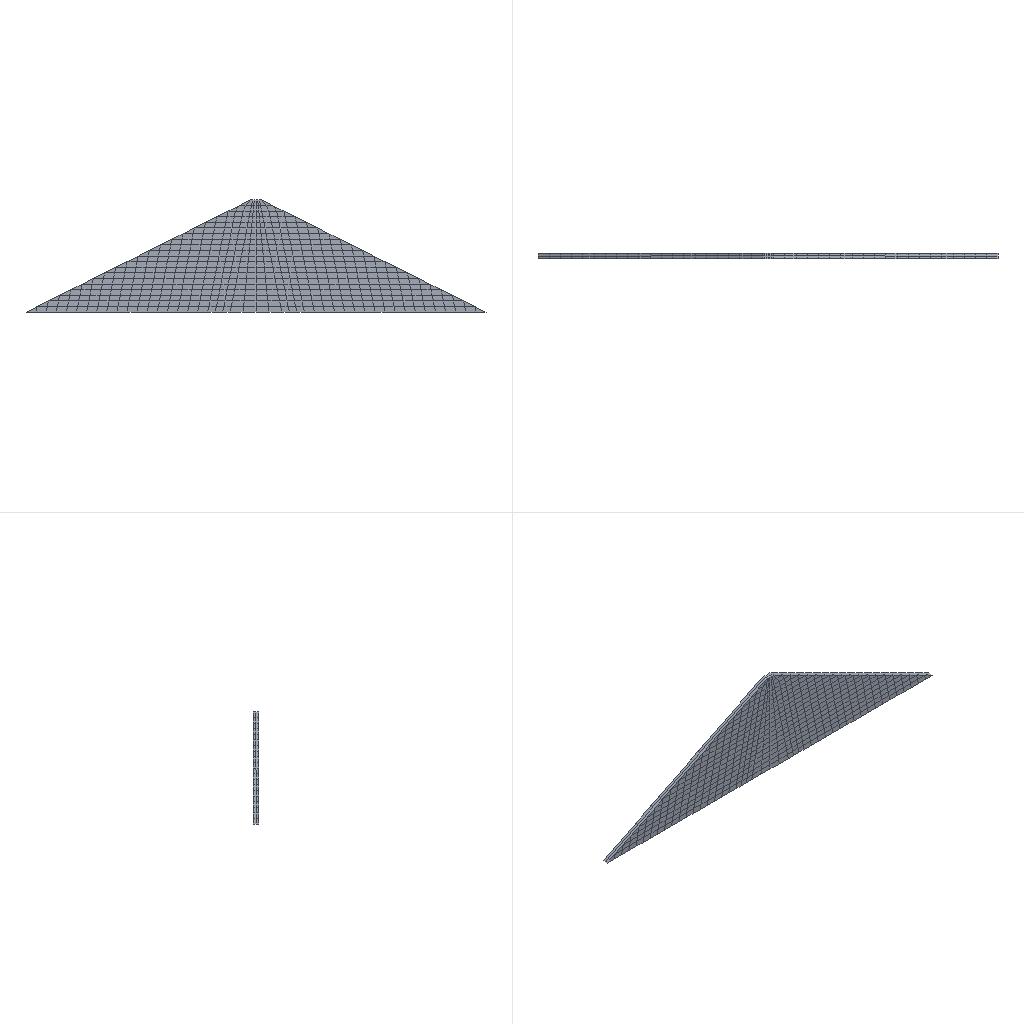Simulation study | abaqus
Set-up summary:
category,name,step,type,value,unit,region
solver,abaqus,,Abaqus/CAE 2024
units,unstated,,unstated,E= density=2 (no match)
analysis,Fill-1,,static,time_period=10
analysis,Fill-2,,static,time_period=10
analysis,Fill-3,,static,time_period=10
analysis,Fill-4,,static,time_period=10
analysis,Fiil-5,,static,time_period=10
analysis,Fill-6,,static,time_period=10
analysis,Fill-7,,static,time_period=10
analysis,Fill-8,,static,time_period=10
analysis,Fill-9,,static,time_period=10
analysis,Fill-10,,static,time_period=10
mesh,nodes,,,1701
mesh,elements,,,1080
element_type,C3D8,,,1000
element_type,C3D6,,,80
material,Core,,density,2
material,Core,,behaviors,depvar; user material
material,Rock,,density,2.2
material,Rock,,behaviors,depvar; user material
section,Rock,,solid section,,,_PickedSet30
section,Core,,solid section,,,_PickedSet29
load,,initial,initial condition solution
load,Load-1,Fill-1,gravity,"10 [dir=(0, 0, -1)]",,Part-1-1.Fill-1
load,Load-2,Fill-2,gravity,"10 [dir=(0, 0, -1)]",,Part-1-1.Fill-2
load,Load-3,Fill-3,gravity,"10 [dir=(0, 0, -1)]",,Part-1-1.Fill-3
load,Load-4,Fill-4,gravity,"10 [dir=(0, 0, -1)]",,Part-1-1.Fill-4
load,Load-5,Fiil-5,gravity,"10 [dir=(0, 0, -1)]",,Part-1-1.Fill-5
load,Load-6,Fill-6,gravity,"10 [dir=(0, 0, -1)]",,Part-1-1.Fill-6
load,Load-7,Fill-7,gravity,"10 [dir=(0, 0, -1)]",,Part-1-1.Fill-7
load,Load-8,Fill-8,gravity,"10 [dir=(0, 0, -1)]",,Part-1-1.Fill-8
load,Load-9,Fill-9,gravity,"10 [dir=(0, 0, -1)]",,Part-1-1.Fill-9
load,Load-10,Fill-10,gravity,"10 [dir=(0, 0, -1)]",,Part-1-1.Fill-10
bc,BC-1,initial,fixed,[dofs=y],,Front
bc,BC-2,initial,fixed,[dofs=y],,Back
bc,BC-3,initial,fixed,"[dofs=x,y,z n=3]",,Bottom
Abaqus input file, long lists of numbers shortened:
*Heading
** Job name: deck Model name: Model-1
** Generated by: Abaqus/CAE 2024
*Preprint, echo=NO, model=NO, history=NO, contact=NO
**
** PARTS
**
*Part, name=Part-1
*Node
      1,   185.009,    9.996,           0.
      2,   187.008,           0.,           0.
** (1699 more lines like these left out)
*Element, type=C3D8
1,  278,  993, 1562,  991,    1,  269,  989,  272
2,  993,  280,  992, 1562,  269,    2,  270,  989
** (998 more lines like these left out)
*Element, type=C3D6
953,  941,    1,  269, 1536,  278,  993
954,  942,  261,  941, 1537,  943, 1536
** (78 more lines like these left out)
*Nset, nset=Rock
    1,    2,    3,    4,    5,    6,    7,    8,    9,   10,   11,   12,   13,   14,   15,   16
   17,   18,   19,   20,   21,   22,   23,   24,   25,   26,   27,   28,   29,   30,   31,   32
** (93 more lines like these left out)
*Elset, elset=Rock
    1,    2,    3,    4,    5,    6,    7,    8,    9,   10,   11,   12,   13,   14,   15,   16
   17,   18,   19,   20,   21,   22,   23,   24,   25,   26,   27,   28,   29,   30,   31,   32
** (56 more lines like these left out)
*Nset, nset=Core
  108,  109,  110,  111,  113,  114,  220,  221,  222,  223,  225,  226,  227,  228,  229,  230
  231,  232,  233,  234,  235,  236,  237,  238,  239,  240,  241,  242,  243,  244,  247,  248
** (18 more lines like these left out)
*Elset, elset=Core
 673, 674, 675, 676, 677, 678, 679, 680, 681, 682, 683, 684, 685, 686, 687, 688
 701, 702, 703, 704, 705, 706, 707, 708, 709, 710, 711, 712, 713, 714, 715, 716
** (8 more lines like these left out)
*Nset, nset=Fill-2
    1,    4,    7,    8,   10,   12,   14,   15,   17,   18,   21,   22,   23,   26,   29,   30
   31,   33,   45,   46,   47,   48,   49,   50,   51,   52,   65,   66,   67,   68,   93,   94
** (22 more lines like these left out)
*Elset, elset=Fill-2
   25,   26,   27,   28,   29,   30,   31,   32,   49,   50,   51,   52,   53,   54,   55,   56
   57,   58,   59,   60,   61,   62,   63,   64,   89,   90,   91,   92,   93,   94,   95,   96
** (9 more lines like these left out)
*Nset, nset=Fill-1
    1,    2,    3,    4,    5,    6,    7,    8,    9,   10,   11,   12,   23,   24,   25,   26
   27,   28,   29,   30,   46,   47,   49,   50,   59,   60,   61,   62,   65,   67,   73,   74
** (24 more lines like these left out)
*Elset, elset=Fill-1
    1,    2,    3,    4,    5,    6,    7,    8,    9,   10,   11,   12,   13,   14,   15,   16
   33,   34,   35,   36,   37,   38,   39,   40,   73,   74,   75,   76,   77,   78,   79,   80
** (10 more lines like these left out)
*Nset, nset=Fill-3
   13,   14,   15,   16,   17,   18,   19,   20,   21,   22,   31,   32,   33,   34,   45,   48
   51,   52,   53,   54,   55,   56,   66,   68,   69,   70,   94,   96,   97,   98,  131,  132
** (19 more lines like these left out)
*Elset, elset=Fill-3
   17,   18,   19,   20,   21,   22,   23,   24,   41,   42,   43,   44,   45,   46,   47,   48
   97,   98,   99,  100,  101,  102,  103,  104,  137,  138,  139,  140,  141,  142,  143,  144
** (8 more lines like these left out)
*Nset, nset=Fill-4
   13,   16,   19,   20,   32,   34,   35,   36,   37,   38,   41,   44,   53,   54,   55,   56
   57,   58,   69,   70,   71,   72,   97,   98,   99,  100,  132,  133,  135,  136,  146,  148
** (17 more lines like these left out)
*Elset, elset=Fill-4
   65,   66,   67,   68,   69,   70,   71,   72,  105,  106,  107,  108,  109,  110,  111,  112
  145,  146,  147,  148,  149,  150,  151,  152,  209,  210,  211,  212,  213,  214,  215,  216
** (7 more lines like these left out)
*Nset, nset=Fill-5
   35,   36,   37,   38,   39,   40,   41,   42,   43,   44,   57,   58,   63,   64,   71,   72
   85,   86,   99,  100,  103,  105,  154,  155,  156,  157,  166,  168,  171,  172,  173,  174
** (15 more lines like these left out)
*Elset, elset=Fill-5
   81,   82,   83,   84,   85,   86,   87,   88,  121,  122,  123,  124,  125,  126,  127,  128
  177,  178,  179,  180,  181,  182,  183,  184,  241,  242,  243,  244,  245,  246,  247,  248
** (6 more lines like these left out)
*Nset, nset=Fill-6
   39,   40,   42,   43,   63,   64,   75,   76,   77,   78,   80,   82,   85,   86,  103,  104
  105,  106,  171,  172,  173,  174,  175,  176,  177,  178,  179,  180,  191,  193,  195,  196
** (13 more lines like these left out)
*Elset, elset=Fill-6
  161,  162,  163,  164,  165,  166,  167,  168,  225,  226,  227,  228,  229,  230,  231,  232
  273,  274,  275,  276,  277,  278,  279,  280,  457,  458,  459,  460,  461,  462,  463,  464
** (5 more lines like these left out)
*Nset, nset=Fill-7
   75,   76,   77,   78,   79,   80,   81,   82,   83,   84,   88,   90,  104,  106,  113,  114
  177,  178,  179,  180,  197,  198,  199,  200,  209,  210,  211,  212,  215,  218,  229,  230
** (10 more lines like these left out)
*Elset, elset=Fill-7
  169,  170,  171,  172,  173,  174,  175,  176,  233,  234,  235,  236,  237,  238,  239,  240
  545,  546,  547,  548,  549,  550,  551,  552,  585,  586,  587,  588,  589,  590,  591,  592
** (4 more lines like these left out)
*Nset, nset=Fill-8
   79,   81,   83,   84,   87,   88,   89,   90,   91,   92,  108,  110,  113,  114,  209,  210
  211,  212,  213,  214,  215,  216,  217,  218,  220,  222,  255,  256,  429,  433,  434,  435
** (8 more lines like these left out)
*Elset, elset=Fill-8
  185,  186,  187,  188,  189,  190,  191,  192,  261,  262,  263,  264,  265,  266,  267,  268
  269,  270,  271,  272,  553,  554,  555,  556,  557,  558,  559,  560,  857,  858,  859,  860
** (3 more lines like these left out)
*Nset, nset=Fill-9
   87,   89,   91,   92,  107,  108,  109,  110,  111,  112,  213,  214,  216,  217,  219,  220
  221,  222,  223,  224,  445,  449,  450,  451,  490,  491,  492,  493,  494,  495,  496,  497
** (6 more lines like these left out)
*Elset, elset=Fill-9
  249,  250,  251,  252,  253,  254,  255,  256,  257,  258,  259,  260,  561,  562,  563,  564
  565,  566,  567,  568,  569,  570,  571,  572,  937,  938,  939,  940,  941,  942,  943,  944
** (2 more lines like these left out)
*Nset, nset=Fill-10
  107,  109,  111,  112,  219,  221,  223,  224,  257,  258,  259,  260,  265,  266,  267,  268
  494,  495,  500,  501,  502,  503,  744,  745,  750,  751,  752,  753,  923,  924,  925,  926
** (4 more lines like these left out)
*Elset, elset=Fill-10
  921,  922,  923,  924,  925,  926,  927,  928,  929,  930,  931,  932,  933,  934,  935,  936
 1049, 1050, 1051, 1052, 1053, 1054, 1055, 1056, 1057, 1058, 1059, 1060, 1061, 1062, 1063, 1064
** (1 more lines like these left out)
*Nset, nset=_PickedSet29, internal
  108,  109,  110,  111,  113,  114,  220,  221,  222,  223,  225,  226,  227,  228,  229,  230
  231,  232,  233,  234,  235,  236,  237,  238,  239,  240,  241,  242,  243,  244,  247,  248
** (18 more lines like these left out)
*Elset, elset=_PickedSet29, internal
 673, 674, 675, 676, 677, 678, 679, 680, 681, 682, 683, 684, 685, 686, 687, 688
 701, 702, 703, 704, 705, 706, 707, 708, 709, 710, 711, 712, 713, 714, 715, 716
** (8 more lines like these left out)
*Nset, nset=_PickedSet30, internal
    1,    2,    3,    4,    5,    6,    7,    8,    9,   10,   11,   12,   13,   14,   15,   16
   17,   18,   19,   20,   21,   22,   23,   24,   25,   26,   27,   28,   29,   30,   31,   32
** (93 more lines like these left out)
*Elset, elset=_PickedSet30, internal
    1,    2,    3,    4,    5,    6,    7,    8,    9,   10,   11,   12,   13,   14,   15,   16
   17,   18,   19,   20,   21,   22,   23,   24,   25,   26,   27,   28,   29,   30,   31,   32
** (56 more lines like these left out)
*Nset, nset=all, generate
    1,  1701,     1
*Elset, elset=all, generate
    1,  1080,     1
** Section: rock
*Solid Section, elset=_PickedSet30, material=Rock
1.,
** Section: core
*Solid Section, elset=_PickedSet29, material=Core
1.,
*End Part
**
**
** ASSEMBLY
**
*Assembly, name=Assembly
**
*Instance, name=Part-1-1, part=Part-1
          0.,           0.,           0.
          0.,           0.,           0., 1.,           0.,           0., 90.
*End Instance
**
*Nset, nset=Back, instance=Part-1-1
    1,    2,    3,    4,    9,   10,   13,   14,   15,   16,   22,   23,   24,   25,   26,   31
   32,   37,   38,   42,   43,   44,   45,   46,   47,   48,   53,   54,   57,   59,   60,   64
** (34 more lines like these left out)
*Elset, elset=Back, instance=Part-1-1
    1,    2,    3,    4,    9,   10,   11,   12,   17,   18,   19,   20,   29,   30,   31,   32
   33,   34,   35,   36,   41,   42,   43,   44,   49,   50,   51,   52,   61,   62,   63,   64
** (32 more lines like these left out)
*Nset, nset=Bottom, instance=Part-1-1
    2,    3,    5,    6,    9,   11,   24,   25,   27,   28,   59,   60,   61,   62,   73,   74
  101,  102,  115,  118,  121,  122,  123,  124,  128,  130,  142,  144,  150,  152,  162,  164
** (7 more lines like these left out)
*Elset, elset=Bottom, instance=Part-1-1
    2,    4,    6,    8,   10,   12,   14,   16,   34,   36,   38,   40,   73,   75,   77,   79
  114,  116,  118,  120,  154,  156,  158,  160,  218,  220,  222,  224,  281,  283,  285,  287
** (4 more lines like these left out)
*Nset, nset=Front, instance=Part-1-1
    5,    6,    7,    8,   11,   12,   17,   18,   19,   20,   21,   27,   28,   29,   30,   33
   34,   35,   36,   39,   40,   41,   49,   50,   51,   52,   55,   56,   58,   61,   62,   63
** (34 more lines like these left out)
*Elset, elset=Front, instance=Part-1-1
    5,    6,    7,    8,   13,   14,   15,   16,   21,   22,   23,   24,   25,   26,   27,   28
   37,   38,   39,   40,   45,   46,   47,   48,   53,   54,   55,   56,   57,   58,   59,   60
** (32 more lines like these left out)
*End Assembly
**
** MATERIALS
**
*Material, name=Core
*Density
2.,
*Depvar
      3,
*User Material, constants=10
500., 0.35,  0.8,  50.,  30.,   0., 470., 0.15
 800., 100.
*Material, name=Rock
*Density
 2.2,
*Depvar
      3,
*User Material, constants=10
1100.,  0.3,  0.8,  10.,  40.,   0., 600.,  0.1
1800., 100.
**
** BOUNDARY CONDITIONS
**
** Name: BC-1 Type: Displacement/Rotation
*Boundary
Front, 2, 2
** Name: BC-2 Type: Displacement/Rotation
*Boundary
Back, 2, 2
** Name: BC-3 Type: Displacement/Rotation
*Boundary
Bottom, 1, 1
Bottom, 2, 2
Bottom, 3, 3
** ----------------------------------------------------------------
*initial conditions,type=solution
part-1-1.all,0,100,0
**
** STEP: Fill-1
**
*Step, name=Fill-1, nlgeom=NO
*Static
1., 10., 0.0001, 1.
**
** LOADS
**
** Name: Load-1   Type: Gravity
*Dload
Part-1-1.Fill-1, GRAV, 10., 0., 0., -1.
**
** INTERACTIONS
**
** Interaction: Int-1
*Model Change, remove
Part-1-1.Fill-2,
** Interaction: Int-2
*Model Change, remove
Part-1-1.Fill-3,
** Interaction: Int-3
*Model Change, remove
Part-1-1.Fill-4,
** Interaction: Int-4
*Model Change, remove
Part-1-1.Fill-5,
** Interaction: Int-5
*Model Change, remove
Part-1-1.Fill-6,
** Interaction: Int-6
*Model Change, remove
Part-1-1.Fill-7,
** Interaction: Int-7
*Model Change, remove
Part-1-1.Fill-8,
** Interaction: Int-8
*Model Change, remove
Part-1-1.Fill-9,
** Interaction: Int-9
*Model Change, remove
Part-1-1.Fill-10,
**
** OUTPUT REQUESTS
**
*Restart, write, frequency=0
*Print, solve=NO
**
** FIELD OUTPUT: F-Output-1
**
*Output, field
*Node Output
COORD, U
*Element Output, directions=YES
COORD, E, S, SDV
**
** HISTORY OUTPUT: H-Output-1
**
*Output, history, variable=PRESELECT
*End Step
** ----------------------------------------------------------------
**
** STEP: Fill-2
**
*Step, name=Fill-2, nlgeom=NO
*Static
1., 10., 0.0001, 1.
**
** LOADS
**
** Name: Load-2   Type: Gravity
*Dload
Part-1-1.Fill-2, GRAV, 10., 0., 0., -1.
**
** INTERACTIONS
**
** Interaction: Int-1
*Model Change, add
Part-1-1.Fill-2,
**
** OUTPUT REQUESTS
**
*Restart, write, frequency=0
**
** FIELD OUTPUT: F-Output-1
**
*Output, field
*Node Output
COORD, U
*Element Output, directions=YES
COORD, E, S, SDV
**
** HISTORY OUTPUT: H-Output-1
**
*Output, history, variable=PRESELECT
*End Step
** ----------------------------------------------------------------
**
** STEP: Fill-3
**
*Step, name=Fill-3, nlgeom=NO
*Static
1., 10., 0.0001, 1.
**
** LOADS
**
** Name: Load-3   Type: Gravity
*Dload
Part-1-1.Fill-3, GRAV, 10., 0., 0., -1.
**
** INTERACTIONS
**
** Interaction: Int-2
*Model Change, add
Part-1-1.Fill-3,
**
** OUTPUT REQUESTS
**
*Restart, write, frequency=0
**
** FIELD OUTPUT: F-Output-1
**
*Output, field
*Node Output
COORD, U
*Element Output, directions=YES
COORD, E, S, SDV
**
** HISTORY OUTPUT: H-Output-1
**
*Output, history, variable=PRESELECT
*End Step
** ----------------------------------------------------------------
**
** STEP: Fill-4
**
*Step, name=Fill-4, nlgeom=NO
*Static
1., 10., 0.0001, 1.
**
** LOADS
**
** Name: Load-4   Type: Gravity
*Dload
Part-1-1.Fill-4, GRAV, 10., 0., 0., -1.
**
** INTERACTIONS
**
** Interaction: Int-3
*Model Change, add
Part-1-1.Fill-4,
**
** OUTPUT REQUESTS
**
*Restart, write, frequency=0
**
** FIELD OUTPUT: F-Output-1
**
*Output, field
*Node Output
COORD, U
*Element Output, directions=YES
COORD, E, S, SDV
**
** HISTORY OUTPUT: H-Output-1
**
*Output, history, variable=PRESELECT
*End Step
** ----------------------------------------------------------------
**
** STEP: Fiil-5
**
*Step, name=Fiil-5, nlgeom=NO
*Static
1., 10., 0.0001, 1.
**
** LOADS
**
** Name: Load-5   Type: Gravity
*Dload
Part-1-1.Fill-5, GRAV, 10., 0., 0., -1.
**
** INTERACTIONS
**
** Interaction: Int-4
*Model Change, add
Part-1-1.Fill-5,
**
** OUTPUT REQUESTS
**
*Restart, write, frequency=0
**
** FIELD OUTPUT: F-Output-1
**
*Output, field
*Node Output
COORD, U
*Element Output, directions=YES
COORD, E, S, SDV
**
** HISTORY OUTPUT: H-Output-1
**
*Output, history, variable=PRESELECT
*End Step
** ----------------------------------------------------------------
**
** STEP: Fill-6
**
*Step, name=Fill-6, nlgeom=NO
*Static
1., 10., 0.0001, 1.
**
** LOADS
**
** Name: Load-6   Type: Gravity
*Dload
Part-1-1.Fill-6, GRAV, 10., 0., 0., -1.
**
** INTERACTIONS
**
** Interaction: Int-5
*Model Change, add
Part-1-1.Fill-6,
**
** OUTPUT REQUESTS
**
*Restart, write, frequency=0
**
** FIELD OUTPUT: F-Output-1
**
*Output, field
*Node Output
COORD, U
*Element Output, directions=YES
COORD, E, S, SDV
**
** HISTORY OUTPUT: H-Output-1
**
*Output, history, variable=PRESELECT
*End Step
** ----------------------------------------------------------------
**
** STEP: Fill-7
**
*Step, name=Fill-7, nlgeom=NO
*Static
1., 10., 0.0001, 1.
**
** LOADS
**
** Name: Load-7   Type: Gravity
*Dload
Part-1-1.Fill-7, GRAV, 10., 0., 0., -1.
**
** INTERACTIONS
**
** Interaction: Int-6
*Model Change, add
Part-1-1.Fill-7,
**
** OUTPUT REQUESTS
**
*Restart, write, frequency=0
**
** FIELD OUTPUT: F-Output-1
**
*Output, field
*Node Output
COORD, U
*Element Output, directions=YES
COORD, E, S, SDV
**
** HISTORY OUTPUT: H-Output-1
**
*Output, history, variable=PRESELECT
*End Step
** ----------------------------------------------------------------
**
** STEP: Fill-8
**
*Step, name=Fill-8, nlgeom=NO
*Static
1., 10., 0.0001, 1.
**
** LOADS
**
** Name: Load-8   Type: Gravity
*Dload
Part-1-1.Fill-8, GRAV, 10., 0., 0., -1.
**
** INTERACTIONS
**
** Interaction: Int-7
*Model Change, add
Part-1-1.Fill-8,
**
** OUTPUT REQUESTS
**
*Restart, write, frequency=0
**
** FIELD OUTPUT: F-Output-1
**
*Output, field
*Node Output
COORD, U
*Element Output, directions=YES
COORD, E, S, SDV
**
** HISTORY OUTPUT: H-Output-1
**
*Output, history, variable=PRESELECT
*End Step
** ----------------------------------------------------------------
**
** STEP: Fill-9
**
*Step, name=Fill-9, nlgeom=NO
*Static
1., 10., 0.0001, 1.
**
** LOADS
**
** Name: Load-9   Type: Gravity
*Dload
Part-1-1.Fill-9, GRAV, 10., 0., 0., -1.
**
** INTERACTIONS
**
** Interaction: Int-8
*Model Change, add
Part-1-1.Fill-9,
**
** OUTPUT REQUESTS
**
*Restart, write, frequency=0
**
** FIELD OUTPUT: F-Output-1
**
*Output, field
*Node Output
COORD, U
*Element Output, directions=YES
COORD, E, S, SDV
**
** HISTORY OUTPUT: H-Output-1
**
*Output, history, variable=PRESELECT
*End Step
** ----------------------------------------------------------------
**
** STEP: Fill-10
**
*Step, name=Fill-10, nlgeom=NO
*Static
1., 10., 0.0001, 1.
**
** LOADS
**
** Name: Load-10   Type: Gravity
*Dload
Part-1-1.Fill-10, GRAV, 10., 0., 0., -1.
**
** INTERACTIONS
**
** Interaction: Int-9
*Model Change, add
Part-1-1.Fill-10,
**
** OUTPUT REQUESTS
**
*Restart, write, frequency=0
**
** FIELD OUTPUT: F-Output-1
**
*Output, field
*Node Output
COORD, U
*Element Output, directions=YES
COORD, E, S, SDV
**
** HISTORY OUTPUT: H-Output-1
**
*Output, history, variable=PRESELECT
*End Step
Results summary, first 50 of 91 lines:
result,odb.job_status,,,JOB_STATUS_COMPLETED_SUCCESSFULLY,"consistent, unstated (Abaqus has no unit system)"
result,steps[0].procedure,Fill-1,,*STATIC,"consistent, unstated (Abaqus has no unit system)"
result,steps[0].time_period,Fill-1,,10,"consistent, unstated (Abaqus has no unit system)"
result,steps[0].n_frames,Fill-1,,11,"consistent, unstated (Abaqus has no unit system)"
result,steps[0].last_frame.id,Fill-1,,10,"consistent, unstated (Abaqus has no unit system)"
result,steps[0].last_frame.value,Fill-1,,10,"consistent, unstated (Abaqus has no unit system)"
result,steps[0].last_frame.description,Fill-1,,Increment     10: Step Time =    10.00,"consistent, unstated (Abaqus has no unit system)"
result,steps[0].completed,Fill-1,,True,"consistent, unstated (Abaqus has no unit system)"
result,steps[0].max_U_magnitude,Fill-1,,0.0153,"consistent, unstated (Abaqus has no unit system)"
result,steps[0].max_S_mises,Fill-1,,100.194,"consistent, unstated (Abaqus has no unit system)"
result,steps[1].procedure,Fill-2,,*STATIC,"consistent, unstated (Abaqus has no unit system)"
result,steps[1].time_period,Fill-2,,10,"consistent, unstated (Abaqus has no unit system)"
result,steps[1].n_frames,Fill-2,,13,"consistent, unstated (Abaqus has no unit system)"
result,steps[1].last_frame.id,Fill-2,,12,"consistent, unstated (Abaqus has no unit system)"
result,steps[1].last_frame.value,Fill-2,,10,"consistent, unstated (Abaqus has no unit system)"
result,steps[1].last_frame.description,Fill-2,,Increment     12: Step Time =    10.00,"consistent, unstated (Abaqus has no unit system)"
result,steps[1].completed,Fill-2,,True,"consistent, unstated (Abaqus has no unit system)"
result,steps[1].max_U_magnitude,Fill-2,,0.04637,"consistent, unstated (Abaqus has no unit system)"
result,steps[1].max_S_mises,Fill-2,,233.116,"consistent, unstated (Abaqus has no unit system)"
result,steps[2].procedure,Fill-3,,*STATIC,"consistent, unstated (Abaqus has no unit system)"
result,steps[2].time_period,Fill-3,,10,"consistent, unstated (Abaqus has no unit system)"
result,steps[2].n_frames,Fill-3,,11,"consistent, unstated (Abaqus has no unit system)"
result,steps[2].last_frame.id,Fill-3,,10,"consistent, unstated (Abaqus has no unit system)"
result,steps[2].last_frame.value,Fill-3,,10,"consistent, unstated (Abaqus has no unit system)"
result,steps[2].last_frame.description,Fill-3,,Increment     10: Step Time =    10.00,"consistent, unstated (Abaqus has no unit system)"
result,steps[2].completed,Fill-3,,True,"consistent, unstated (Abaqus has no unit system)"
result,steps[2].max_U_magnitude,Fill-3,,0.1063,"consistent, unstated (Abaqus has no unit system)"
result,steps[2].max_S_mises,Fill-3,,377.184,"consistent, unstated (Abaqus has no unit system)"
result,steps[3].procedure,Fill-4,,*STATIC,"consistent, unstated (Abaqus has no unit system)"
result,steps[3].time_period,Fill-4,,10,"consistent, unstated (Abaqus has no unit system)"
result,steps[3].n_frames,Fill-4,,11,"consistent, unstated (Abaqus has no unit system)"
result,steps[3].last_frame.id,Fill-4,,10,"consistent, unstated (Abaqus has no unit system)"
result,steps[3].last_frame.value,Fill-4,,10,"consistent, unstated (Abaqus has no unit system)"
result,steps[3].last_frame.description,Fill-4,,Increment     10: Step Time =    10.00,"consistent, unstated (Abaqus has no unit system)"
result,steps[3].completed,Fill-4,,True,"consistent, unstated (Abaqus has no unit system)"
result,steps[3].max_U_magnitude,Fill-4,,0.1603,"consistent, unstated (Abaqus has no unit system)"
result,steps[3].max_S_mises,Fill-4,,526.383,"consistent, unstated (Abaqus has no unit system)"
result,steps[4].procedure,Fiil-5,,*STATIC,"consistent, unstated (Abaqus has no unit system)"
result,steps[4].time_period,Fiil-5,,10,"consistent, unstated (Abaqus has no unit system)"
result,steps[4].n_frames,Fiil-5,,13,"consistent, unstated (Abaqus has no unit system)"
result,steps[4].last_frame.id,Fiil-5,,12,"consistent, unstated (Abaqus has no unit system)"
result,steps[4].last_frame.value,Fiil-5,,10,"consistent, unstated (Abaqus has no unit system)"
result,steps[4].last_frame.description,Fiil-5,,Increment     12: Step Time =    10.00,"consistent, unstated (Abaqus has no unit system)"
result,steps[4].completed,Fiil-5,,True,"consistent, unstated (Abaqus has no unit system)"
result,steps[4].max_U_magnitude,Fiil-5,,0.2385,"consistent, unstated (Abaqus has no unit system)"
result,steps[4].max_S_mises,Fiil-5,,677.558,"consistent, unstated (Abaqus has no unit system)"
result,steps[5].procedure,Fill-6,,*STATIC,"consistent, unstated (Abaqus has no unit system)"
result,steps[5].time_period,Fill-6,,10,"consistent, unstated (Abaqus has no unit system)"
result,steps[5].n_frames,Fill-6,,11,"consistent, unstated (Abaqus has no unit system)"
result,steps[5].last_frame.id,Fill-6,,10,"consistent, unstated (Abaqus has no unit system)"